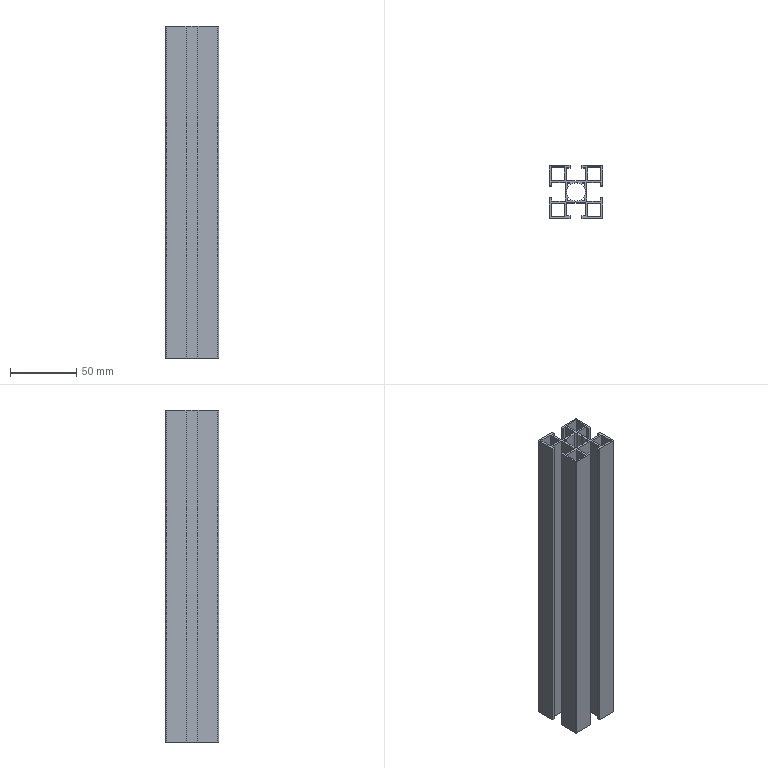Part | 1 solid | 77 faces | box 40 x 40 x 250 mm | volume 99098 mm3 | plane 62 | cylinder 15 | commonest cylinder face diameters 2.2 x6 14 x5 1 x4